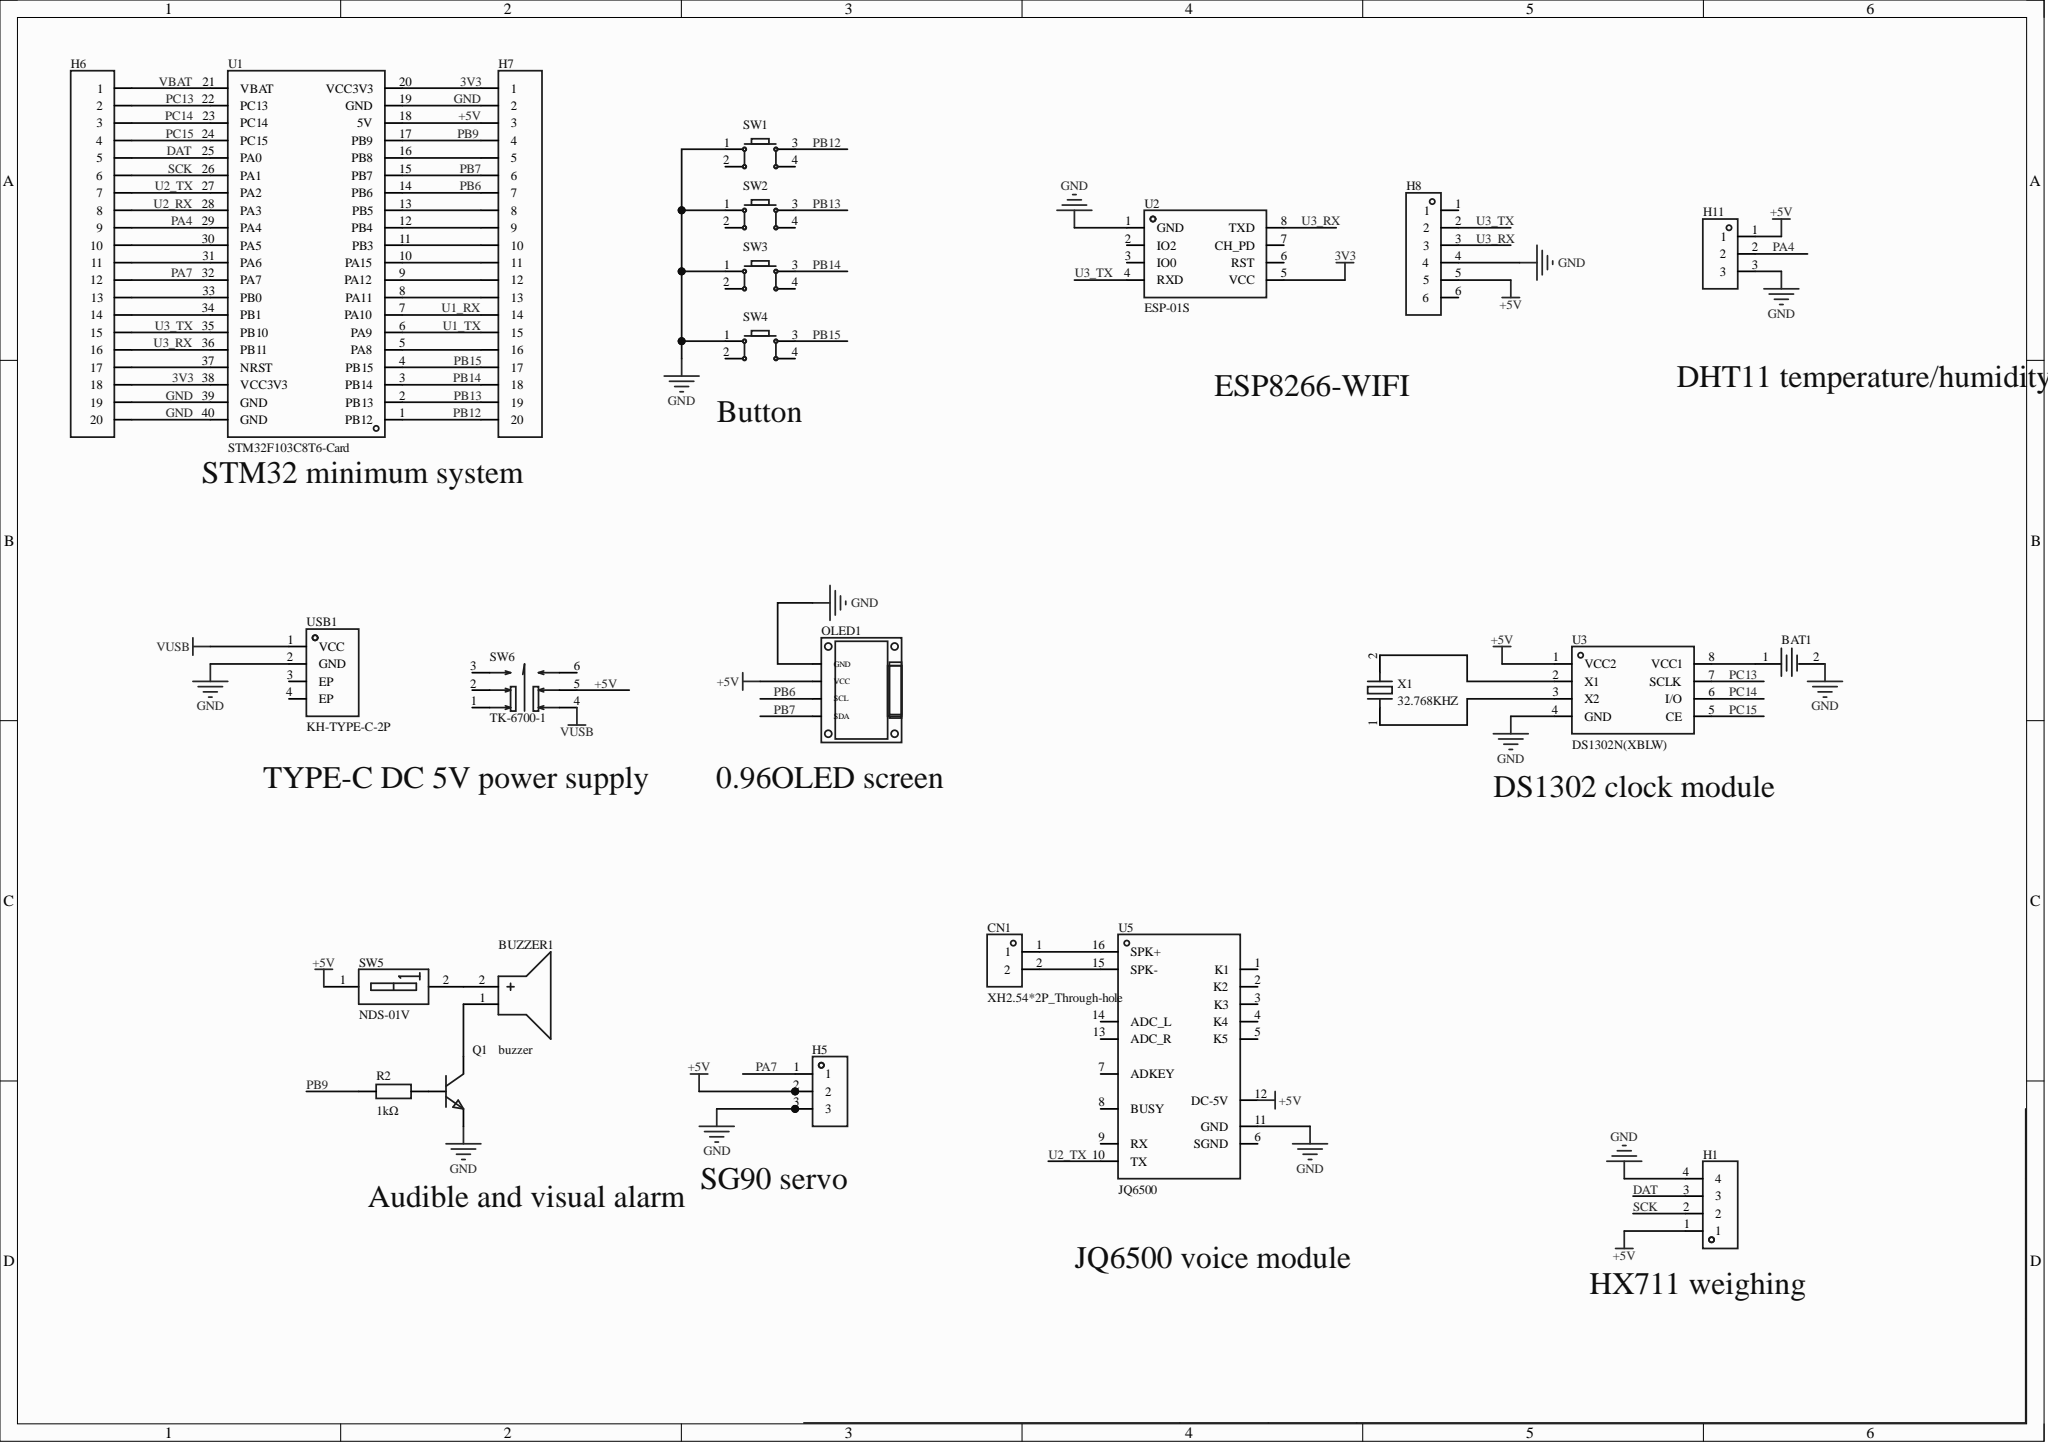Circuit board | Altium Designer | 24 parts | 46 nets
Bill of materials:
Comment,Description,Designator,Footprint,LibRef,Quantity
"KH-BS2032-2-1","","BAT1","BAT-TH_KH-BS2032-2-1","KH-BS2032-2-1","1"
"buzzer","","BUZZER1","BUZ-TH_BD12.0-P6.00-D0.9-RD","buzzer","1"
"XH2.54*2P_Through-hole","","CN1","CONN-TH_2P-P2.50-XH2.54-2P","XH2.54*2P_直插","1"
"","","H1","HDR-TH_4P-P2.54-V-F","HDR-F_2.54_1x4P","1"
"","","H5, H11","HDR-TH_3P-P2.54-V-F","HDR-F_2.54_1x3P","2"
"","","H6, H7","HDR-TH_20P-P2.54-V-F","HDR-F_2.54_1x20P","2"
"","","H8","HDR-TH_6P-P2.54-V-F","HDR-F_2.54_1x6P","1"
"","","OLED1","0.96OLED_4P","0.96OLED模块_4P","1"
"","","Q1","S8050_TO_92","S8050_TO_NPN","1"
"1kΩ","","R2","Res_1/8W","Res_AXIAL-1/8W","1"
"","","SW1, SW2, SW3, SW4","SW-TH_4P-L6.0-W6.0-P4.50-LS6.5","Key_TH_6x6x6","4"
"NDS-01V","Forward toggle, high lever","SW5","SW-TH_2P-L3.9-W9.9-P2.54-LS7.6","NDS-01V_C501305","1"
"TK-6700-1","Circuit:DPDT;Self-lock/No-lock:Self-lock;Mounting:Through-hole;Actuating force:2.3N;Operating life:-;","SW6","SW-TH_TK-6700-1","TK-6700-1","1"
"STM32F103C8T6-Card","","U1","CONN-TH_L53.3-W22.9_STM32F103C8T6-CARD","STM32F103C8T6-Card","1"
"ESP-01S","","U2","WIFIM-TH_ESP-01S","ESP-01S_C111009","1"
"DS1302N(XBLW)","Interface type:Three-wire serial interface;Crystal:External;Alarm output:-;","U3","PDIP-8_L9.3-W6.4-P2.54-LS7.6-BL","DS1302N(XBLW)","1"
"JQ6500","","U5","MOD-TH_JQ6500","JQ6500","1"
"KH-TYPE-C-2P","Connector type:Type-C;Protocol standard:-;Gender:-;Mounting:Right angle;Contacts:2P;Ports:1;Rated current - power:3A;Operating temperature:-25℃~+85℃;","USB1","USB-SMD_KH-TYPE-C-2P","KH-TYPE-C-2P","1"
"32.768KHZ","","X1","CRYSTAL-SMD_L3.2-W1.5-1","32.768KHZ","1"
Netlist (Protel format):
[
BAT1
BAT-TH_KH-BS2032-2-1
KH-BS2032-2-1



]
[
BUZZER1
BUZ-TH_BD12.0-P6.00-D0.9-RD
buzzer



]
[
CN1
CONN-TH_2P-P2.50-XH2.54-2P
XH2.54*2P_Through-hole



]
[
H1
HDR-TH_4P-P2.54-V-F




]
[
H5
HDR-TH_3P-P2.54-V-F




]
[
H6
HDR-TH_20P-P2.54-V-F




]
[
H7
HDR-TH_20P-P2.54-V-F




]
[
H8
HDR-TH_6P-P2.54-V-F




]
[
H11
HDR-TH_3P-P2.54-V-F




]
[
OLED1
0.96OLED_4P




]
[
Q1
S8050_TO_92




]
[
R2
Res_1/8W
1kΩ



]
[
SW1
SW-TH_4P-L6.0-W6.0-P4.50-LS6.5




]
[
SW2
SW-TH_4P-L6.0-W6.0-P4.50-LS6.5




]
[
SW3
SW-TH_4P-L6.0-W6.0-P4.50-LS6.5




]
[
SW4
SW-TH_4P-L6.0-W6.0-P4.50-LS6.5




]
[
SW5
SW-TH_2P-L3.9-W9.9-P2.54-LS7.6
NDS-01V



]
[
SW6
SW-TH_TK-6700-1
TK-6700-1



]
[
U1
CONN-TH_L53.3-W22.9_STM32F103C8T6-CARD
STM32F103C8T6-Card



]
[
U2
WIFIM-TH_ESP-01S
ESP-01S



]
[
U3
PDIP-8_L9.3-W6.4-P2.54-LS7.6-BL
DS1302N(XBLW)



]
[
U5
MOD-TH_JQ6500
JQ6500



]
[
USB1
USB-SMD_KH-TYPE-C-2P
KH-TYPE-C-2P



]
[
X1
CRYSTAL-SMD_L3.2-W1.5-1
32.768KHZ



]
(
VUSB
SW6-4
USB1-1
)
(
VBAT
H6-1
U1-21
)
(
U3_TX
H6-15
H8-2
U1-35
U2-4
)
(
U3_RX
H6-16
H8-3
U1-36
U2-8
)
(
U2_TX
H6-7
U1-27
U5-10
)
(
U2_RX
H6-8
U1-28
)
(
U1_TX
H7-15
U1-6
)
(
U1_RX
H7-14
U1-7
)
(
SCK
H1-2
H6-6
U1-26
)
(
PC15
H6-4
U1-24
U3-5
)
(
PC14
H6-3
U1-23
U3-6
)
(
PC13
H6-2
U1-22
U3-7
)
(
PB15
H7-17
SW4-3
U1-4
)
(
PB14
H7-18
SW3-3
U1-3
)
(
PB13
H7-19
SW2-3
U1-2
)
(
PB12
H7-20
SW1-3
U1-1
)
(
PB9
H7-4
R2-1
U1-17
)
(
PB7
H7-6
OLED1-4
U1-15
)
(
PB6
H7-7
OLED1-3
U1-14
)
(
PA7
H5-1
H6-12
U1-32
)
(
PA4
H6-9
H11-2
U1-29
)
(
NetU3_3
U3-3
X1-1
)
(
NetU3_2
U3-2
X1-2
)
(
NetQ1_2
Q1-2
R2-2
)
(
NetH7_16
H7-16
U1-5
)
(
NetH7_13
H7-13
U1-8
)
(
NetH7_12
H7-12
U1-9
)
(
NetH7_11
H7-11
U1-10
)
(
NetH7_10
H7-10
U1-11
)
(
NetH7_9
H7-9
U1-12
)
(
NetH7_8
H7-8
U1-13
)
(
NetH7_5
H7-5
U1-16
)
(
NetH6_17
H6-17
U1-37
)
(
NetH6_14
H6-14
U1-34
)
(
NetH6_13
H6-13
U1-33
)
(
NetH6_11
H6-11
U1-31
)
(
NetH6_10
H6-10
U1-30
)
(
NetCN1_2
CN1-2
U5-15
)
(
NetCN1_1
CN1-1
U5-16
)
(
NetBUZZER1_2
BUZZER1-2
SW5-2
)
(
NetBUZZER1_1
BUZZER1-1
Q1-3
)
(
NetBAT1_1
BAT1-1
U3-8
)
(
GND
BAT1-2
H1-4
H5-3
H6-19
H6-20
H7-2
H8-4
H11-3
OLED1-1
Q1-1
SW1-1
SW2-1
SW3-1
SW4-1
U1-19
U1-39
U1-40
U2-1
U3-4
U5-11
USB1-2
)
(
DAT
H1-3
H6-5
U1-25
)
(
+5V
H1-1
H5-2
H7-3
H8-5
H11-1
OLED1-2
SW5-1
SW6-5
U1-18
U3-1
U5-12
)
(
3V3
H6-18
H7-1
U1-20
U1-38
U2-5
)